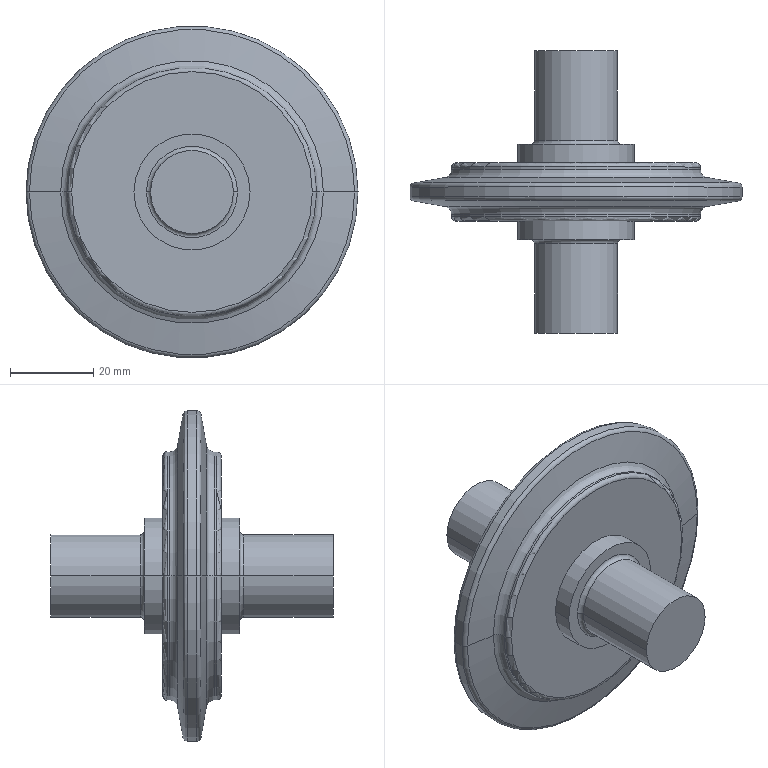Part | SolidWorks | features Revolution 1 | 1 solid | 40 faces | box 80 x 68 x 80 mm | volume 71844 mm3 | torus 16 | cylinder 14 | plane 6 | cone 4 | commonest cylinder face diameters 20 x4 28 x4 60 x4 80 x2
STEP:
#1=CARTESIAN_POINT('',(321.384,33.979,0.));
#2=VERTEX_POINT('',#1);
#3=CARTESIAN_POINT('',(258.079,33.979,0.));
#4=VERTEX_POINT('',#3);
#5=CARTESIAN_POINT('',(289.732,33.979,0.));
#6=DIRECTION('',(0.,-1.,0.));
#7=DIRECTION('',(1.,0.,0.));
#8=AXIS2_PLACEMENT_3D('',#5,#6,#7);
#9=CIRCLE('',#8,31.653);
#10=EDGE_CURVE('',#2,#4,#9,.T.);
#11=ORIENTED_EDGE('',*,*,#10,.T.);
#12=CARTESIAN_POINT('',(250.558,32.653,0.));
#13=VERTEX_POINT('',#12);
#14=CARTESIAN_POINT('',(258.079,33.979,0.));
#15=DIRECTION('',(-0.9848,-0.1736,0.));
#16=VECTOR('',#15,1000.);
#17=LINE('',#14,#16);
#18=EDGE_CURVE('',#4,#13,#17,.T.);
#19=ORIENTED_EDGE('',*,*,#18,.T.);
#20=CARTESIAN_POINT('',(328.905,32.653,0.));
#21=VERTEX_POINT('',#20);
#22=CARTESIAN_POINT('',(289.732,32.653,0.));
#23=DIRECTION('',(0.,-1.,0.));
#24=DIRECTION('',(1.,0.,0.));
#25=AXIS2_PLACEMENT_3D('',#22,#23,#24);
#26=CIRCLE('',#25,39.174);
#27=EDGE_CURVE('',#21,#13,#26,.T.);
#28=ORIENTED_EDGE('',*,*,#27,.F.);
#29=CARTESIAN_POINT('',(321.384,33.979,0.));
#30=DIRECTION('',(0.9848,-0.1736,0.));
#31=VECTOR('',#30,1000.);
#32=LINE('',#29,#31);
#33=EDGE_CURVE('',#2,#21,#32,.T.);
#34=ORIENTED_EDGE('',*,*,#33,.F.);
#35=EDGE_LOOP('',(#11,#19,#28,#34));
#36=FACE_OUTER_BOUND('',#35,.T.);
#37=CARTESIAN_POINT('',(289.732,33.979,0.));
#38=DIRECTION('',(0.,-1.,0.));
#39=DIRECTION('',(1.,0.,0.));
#40=AXIS2_PLACEMENT_3D('',#37,#38,#39);
#41=CONICAL_SURFACE('',#40,31.653,1.396);
#42=ADVANCED_FACE('',(#36),#41,.T.);
#43=CARTESIAN_POINT('',(289.732,33.979,0.));
#44=DIRECTION('',(0.,-1.,0.));
#45=DIRECTION('',(1.,0.,0.));
#46=AXIS2_PLACEMENT_3D('',#43,#44,#45);
#47=CIRCLE('',#46,31.653);
#48=EDGE_CURVE('',#4,#2,#47,.T.);
#49=ORIENTED_EDGE('',*,*,#48,.F.);
#50=CARTESIAN_POINT('',(259.732,35.948,0.));
#51=VERTEX_POINT('',#50);
#52=CARTESIAN_POINT('',(257.732,35.948,0.));
#53=DIRECTION('',(0.,0.,1.));
#54=DIRECTION('',(1.,0.,0.));
#55=AXIS2_PLACEMENT_3D('',#52,#53,#54);
#56=CIRCLE('',#55,2.);
#57=EDGE_CURVE('',#4,#51,#56,.T.);
#58=ORIENTED_EDGE('',*,*,#57,.T.);
#59=CARTESIAN_POINT('',(319.732,35.948,0.));
#60=VERTEX_POINT('',#59);
#61=CARTESIAN_POINT('',(289.732,35.948,0.));
#62=DIRECTION('',(0.,-1.,0.));
#63=DIRECTION('',(1.,0.,0.));
#64=AXIS2_PLACEMENT_3D('',#61,#62,#63);
#65=CIRCLE('',#64,30.);
#66=EDGE_CURVE('',#51,#60,#65,.T.);
#67=ORIENTED_EDGE('',*,*,#66,.T.);
#68=CARTESIAN_POINT('',(321.732,35.948,0.));
#69=DIRECTION('',(0.,0.,-1.));
#70=DIRECTION('',(-1.,0.,0.));
#71=AXIS2_PLACEMENT_3D('',#68,#69,#70);
#72=CIRCLE('',#71,2.);
#73=EDGE_CURVE('',#2,#60,#72,.T.);
#74=ORIENTED_EDGE('',*,*,#73,.F.);
#75=EDGE_LOOP('',(#49,#58,#67,#74));
#76=FACE_OUTER_BOUND('',#75,.T.);
#77=CARTESIAN_POINT('',(289.732,35.948,0.));
#78=DIRECTION('',(0.,-1.,0.));
#79=DIRECTION('',(1.,0.,0.));
#80=AXIS2_PLACEMENT_3D('',#77,#78,#79);
#81=TOROIDAL_SURFACE('',#80,32.,2.);
#82=ADVANCED_FACE('',(#76),#81,.F.);
#83=CARTESIAN_POINT('',(319.732,36.507,0.));
#84=VERTEX_POINT('',#83);
#85=CARTESIAN_POINT('',(259.732,36.507,0.));
#86=VERTEX_POINT('',#85);
#87=CARTESIAN_POINT('',(289.732,36.507,0.));
#88=DIRECTION('',(0.,-1.,0.));
#89=DIRECTION('',(1.,0.,0.));
#90=AXIS2_PLACEMENT_3D('',#87,#88,#89);
#91=CIRCLE('',#90,30.);
#92=EDGE_CURVE('',#84,#86,#91,.T.);
#93=ORIENTED_EDGE('',*,*,#92,.T.);
#94=CARTESIAN_POINT('',(259.732,-3.493,0.));
#95=DIRECTION('',(0.,-1.,0.));
#96=VECTOR('',#95,1000.);
#97=LINE('',#94,#96);
#98=EDGE_CURVE('',#86,#51,#97,.T.);
#99=ORIENTED_EDGE('',*,*,#98,.T.);
#100=CARTESIAN_POINT('',(289.732,35.948,0.));
#101=DIRECTION('',(0.,-1.,0.));
#102=DIRECTION('',(1.,0.,0.));
#103=AXIS2_PLACEMENT_3D('',#100,#101,#102);
#104=CIRCLE('',#103,30.);
#105=EDGE_CURVE('',#60,#51,#104,.T.);
#106=ORIENTED_EDGE('',*,*,#105,.F.);
#107=CARTESIAN_POINT('',(319.732,-3.493,0.));
#108=DIRECTION('',(0.,-1.,0.));
#109=VECTOR('',#108,1000.);
#110=LINE('',#107,#109);
#111=EDGE_CURVE('',#84,#60,#110,.T.);
#112=ORIENTED_EDGE('',*,*,#111,.F.);
#113=EDGE_LOOP('',(#93,#99,#106,#112));
#114=FACE_OUTER_BOUND('',#113,.T.);
#115=CARTESIAN_POINT('',(289.732,-3.493,0.));
#116=DIRECTION('',(0.,-1.,0.));
#117=DIRECTION('',(1.,0.,0.));
#118=AXIS2_PLACEMENT_3D('',#115,#116,#117);
#119=CYLINDRICAL_SURFACE('',#118,30.);
#120=ADVANCED_FACE('',(#114),#119,.T.);
#121=CARTESIAN_POINT('',(318.732,37.507,0.));
#122=VERTEX_POINT('',#121);
#123=CARTESIAN_POINT('',(260.732,37.507,0.));
#124=VERTEX_POINT('',#123);
#125=CARTESIAN_POINT('',(289.732,37.507,0.));
#126=DIRECTION('',(0.,-1.,0.));
#127=DIRECTION('',(1.,0.,0.));
#128=AXIS2_PLACEMENT_3D('',#125,#126,#127);
#129=CIRCLE('',#128,29.);
#130=EDGE_CURVE('',#122,#124,#129,.T.);
#131=ORIENTED_EDGE('',*,*,#130,.T.);
#132=CARTESIAN_POINT('',(260.732,36.507,0.));
#133=DIRECTION('',(0.,0.,1.));
#134=DIRECTION('',(1.,0.,0.));
#135=AXIS2_PLACEMENT_3D('',#132,#133,#134);
#136=CIRCLE('',#135,1.);
#137=EDGE_CURVE('',#124,#86,#136,.T.);
#138=ORIENTED_EDGE('',*,*,#137,.T.);
#139=ORIENTED_EDGE('',*,*,#92,.F.);
#140=CARTESIAN_POINT('',(318.732,36.507,0.));
#141=DIRECTION('',(0.,0.,-1.));
#142=DIRECTION('',(-1.,0.,0.));
#143=AXIS2_PLACEMENT_3D('',#140,#141,#142);
#144=CIRCLE('',#143,1.);
#145=EDGE_CURVE('',#122,#84,#144,.T.);
#146=ORIENTED_EDGE('',*,*,#145,.F.);
#147=EDGE_LOOP('',(#131,#138,#139,#146));
#148=FACE_OUTER_BOUND('',#147,.T.);
#149=CARTESIAN_POINT('',(289.732,36.507,0.));
#150=DIRECTION('',(0.,-1.,0.));
#151=DIRECTION('',(1.,0.,0.));
#152=AXIS2_PLACEMENT_3D('',#149,#150,#151);
#153=TOROIDAL_SURFACE('',#152,29.,1.);
#154=ADVANCED_FACE('',(#148),#153,.T.);
#155=CARTESIAN_POINT('',(303.732,42.007,0.));
#156=VERTEX_POINT('',#155);
#157=CARTESIAN_POINT('',(275.732,42.007,0.));
#158=VERTEX_POINT('',#157);
#159=CARTESIAN_POINT('',(289.732,42.007,0.));
#160=DIRECTION('',(0.,-1.,0.));
#161=DIRECTION('',(1.,0.,0.));
#162=AXIS2_PLACEMENT_3D('',#159,#160,#161);
#163=CIRCLE('',#162,14.);
#164=EDGE_CURVE('',#156,#158,#163,.T.);
#165=ORIENTED_EDGE('',*,*,#164,.T.);
#166=CARTESIAN_POINT('',(275.732,37.507,0.));
#167=VERTEX_POINT('',#166);
#168=CARTESIAN_POINT('',(275.732,-3.493,0.));
#169=DIRECTION('',(0.,-1.,0.));
#170=VECTOR('',#169,1000.);
#171=LINE('',#168,#170);
#172=EDGE_CURVE('',#158,#167,#171,.T.);
#173=ORIENTED_EDGE('',*,*,#172,.T.);
#174=CARTESIAN_POINT('',(303.732,37.507,0.));
#175=VERTEX_POINT('',#174);
#176=CARTESIAN_POINT('',(289.732,37.507,0.));
#177=DIRECTION('',(0.,-1.,0.));
#178=DIRECTION('',(1.,0.,0.));
#179=AXIS2_PLACEMENT_3D('',#176,#177,#178);
#180=CIRCLE('',#179,14.);
#181=EDGE_CURVE('',#175,#167,#180,.T.);
#182=ORIENTED_EDGE('',*,*,#181,.F.);
#183=CARTESIAN_POINT('',(303.732,-3.493,0.));
#184=DIRECTION('',(0.,-1.,0.));
#185=VECTOR('',#184,1000.);
#186=LINE('',#183,#185);
#187=EDGE_CURVE('',#156,#175,#186,.T.);
#188=ORIENTED_EDGE('',*,*,#187,.F.);
#189=EDGE_LOOP('',(#165,#173,#182,#188));
#190=FACE_OUTER_BOUND('',#189,.T.);
#191=CARTESIAN_POINT('',(289.732,-3.493,0.));
#192=DIRECTION('',(0.,-1.,0.));
#193=DIRECTION('',(1.,0.,0.));
#194=AXIS2_PLACEMENT_3D('',#191,#192,#193);
#195=CYLINDRICAL_SURFACE('',#194,14.);
#196=ADVANCED_FACE('',(#190),#195,.T.);
#197=CARTESIAN_POINT('',(278.732,42.007,0.));
#198=VERTEX_POINT('',#197);
#199=CARTESIAN_POINT('',(300.732,42.007,0.));
#200=VERTEX_POINT('',#199);
#201=CARTESIAN_POINT('',(289.732,42.007,0.));
#202=DIRECTION('',(0.,-1.,0.));
#203=DIRECTION('',(1.,0.,0.));
#204=AXIS2_PLACEMENT_3D('',#201,#202,#203);
#205=CIRCLE('',#204,11.);
#206=EDGE_CURVE('',#198,#200,#205,.T.);
#207=ORIENTED_EDGE('',*,*,#206,.F.);
#208=CARTESIAN_POINT('',(279.732,43.007,0.));
#209=VERTEX_POINT('',#208);
#210=CARTESIAN_POINT('',(278.732,43.007,0.));
#211=DIRECTION('',(0.,0.,1.));
#212=DIRECTION('',(1.,0.,0.));
#213=AXIS2_PLACEMENT_3D('',#210,#211,#212);
#214=CIRCLE('',#213,1.);
#215=EDGE_CURVE('',#198,#209,#214,.T.);
#216=ORIENTED_EDGE('',*,*,#215,.T.);
#217=CARTESIAN_POINT('',(299.732,43.007,0.));
#218=VERTEX_POINT('',#217);
#219=CARTESIAN_POINT('',(289.732,43.007,0.));
#220=DIRECTION('',(0.,-1.,0.));
#221=DIRECTION('',(1.,0.,0.));
#222=AXIS2_PLACEMENT_3D('',#219,#220,#221);
#223=CIRCLE('',#222,10.);
#224=EDGE_CURVE('',#209,#218,#223,.T.);
#225=ORIENTED_EDGE('',*,*,#224,.T.);
#226=CARTESIAN_POINT('',(300.732,43.007,0.));
#227=DIRECTION('',(0.,0.,-1.));
#228=DIRECTION('',(-1.,0.,0.));
#229=AXIS2_PLACEMENT_3D('',#226,#227,#228);
#230=CIRCLE('',#229,1.);
#231=EDGE_CURVE('',#200,#218,#230,.T.);
#232=ORIENTED_EDGE('',*,*,#231,.F.);
#233=EDGE_LOOP('',(#207,#216,#225,#232));
#234=FACE_OUTER_BOUND('',#233,.T.);
#235=CARTESIAN_POINT('',(289.732,43.007,0.));
#236=DIRECTION('',(0.,-1.,0.));
#237=DIRECTION('',(1.,0.,0.));
#238=AXIS2_PLACEMENT_3D('',#235,#236,#237);
#239=TOROIDAL_SURFACE('',#238,11.,1.);
#240=ADVANCED_FACE('',(#234),#239,.F.);
#241=CARTESIAN_POINT('',(299.732,64.507,0.));
#242=VERTEX_POINT('',#241);
#243=CARTESIAN_POINT('',(279.732,64.507,0.));
#244=VERTEX_POINT('',#243);
#245=CARTESIAN_POINT('',(289.732,64.507,0.));
#246=DIRECTION('',(0.,-1.,0.));
#247=DIRECTION('',(1.,0.,0.));
#248=AXIS2_PLACEMENT_3D('',#245,#246,#247);
#249=CIRCLE('',#248,10.);
#250=EDGE_CURVE('',#242,#244,#249,.T.);
#251=ORIENTED_EDGE('',*,*,#250,.T.);
#252=CARTESIAN_POINT('',(279.732,-3.493,0.));
#253=DIRECTION('',(0.,-1.,0.));
#254=VECTOR('',#253,1000.);
#255=LINE('',#252,#254);
#256=EDGE_CURVE('',#244,#209,#255,.T.);
#257=ORIENTED_EDGE('',*,*,#256,.T.);
#258=CARTESIAN_POINT('',(289.732,43.007,0.));
#259=DIRECTION('',(0.,-1.,0.));
#260=DIRECTION('',(1.,0.,0.));
#261=AXIS2_PLACEMENT_3D('',#258,#259,#260);
#262=CIRCLE('',#261,10.);
#263=EDGE_CURVE('',#218,#209,#262,.T.);
#264=ORIENTED_EDGE('',*,*,#263,.F.);
#265=CARTESIAN_POINT('',(299.732,-3.493,0.));
#266=DIRECTION('',(0.,-1.,0.));
#267=VECTOR('',#266,1000.);
#268=LINE('',#265,#267);
#269=EDGE_CURVE('',#242,#218,#268,.T.);
#270=ORIENTED_EDGE('',*,*,#269,.F.);
#271=EDGE_LOOP('',(#251,#257,#264,#270));
#272=FACE_OUTER_BOUND('',#271,.T.);
#273=CARTESIAN_POINT('',(289.732,-3.493,0.));
#274=DIRECTION('',(0.,-1.,0.));
#275=DIRECTION('',(1.,0.,0.));
#276=AXIS2_PLACEMENT_3D('',#273,#274,#275);
#277=CYLINDRICAL_SURFACE('',#276,10.);
#278=ADVANCED_FACE('',(#272),#277,.T.);
#279=CARTESIAN_POINT('',(299.732,18.007,0.));
#280=VERTEX_POINT('',#279);
#281=CARTESIAN_POINT('',(279.732,18.007,0.));
#282=VERTEX_POINT('',#281);
#283=CARTESIAN_POINT('',(289.732,18.007,0.));
#284=DIRECTION('',(0.,-1.,0.));
#285=DIRECTION('',(1.,0.,0.));
#286=AXIS2_PLACEMENT_3D('',#283,#284,#285);
#287=CIRCLE('',#286,10.);
#288=EDGE_CURVE('',#280,#282,#287,.T.);
#289=ORIENTED_EDGE('',*,*,#288,.T.);
#290=CARTESIAN_POINT('',(279.732,-3.493,0.));
#291=VERTEX_POINT('',#290);
#292=CARTESIAN_POINT('',(279.732,-3.493,0.));
#293=DIRECTION('',(0.,-1.,0.));
#294=VECTOR('',#293,1000.);
#295=LINE('',#292,#294);
#296=EDGE_CURVE('',#282,#291,#295,.T.);
#297=ORIENTED_EDGE('',*,*,#296,.T.);
#298=CARTESIAN_POINT('',(299.732,-3.493,0.));
#299=VERTEX_POINT('',#298);
#300=CARTESIAN_POINT('',(289.732,-3.493,0.));
#301=DIRECTION('',(0.,-1.,0.));
#302=DIRECTION('',(1.,0.,0.));
#303=AXIS2_PLACEMENT_3D('',#300,#301,#302);
#304=CIRCLE('',#303,10.);
#305=EDGE_CURVE('',#299,#291,#304,.T.);
#306=ORIENTED_EDGE('',*,*,#305,.F.);
#307=CARTESIAN_POINT('',(299.732,-3.493,0.));
#308=DIRECTION('',(0.,-1.,0.));
#309=VECTOR('',#308,1000.);
#310=LINE('',#307,#309);
#311=EDGE_CURVE('',#280,#299,#310,.T.);
#312=ORIENTED_EDGE('',*,*,#311,.F.);
#313=EDGE_LOOP('',(#289,#297,#306,#312));
#314=FACE_OUTER_BOUND('',#313,.T.);
#315=CARTESIAN_POINT('',(289.732,-3.493,0.));
#316=DIRECTION('',(0.,-1.,0.));
#317=DIRECTION('',(1.,0.,0.));
#318=AXIS2_PLACEMENT_3D('',#315,#316,#317);
#319=CYLINDRICAL_SURFACE('',#318,10.);
#320=ADVANCED_FACE('',(#314),#319,.T.);
#321=CARTESIAN_POINT('',(289.732,18.007,0.));
#322=DIRECTION('',(0.,-1.,0.));
#323=DIRECTION('',(1.,0.,0.));
#324=AXIS2_PLACEMENT_3D('',#321,#322,#323);
#325=CIRCLE('',#324,10.);
#326=EDGE_CURVE('',#282,#280,#325,.T.);
#327=ORIENTED_EDGE('',*,*,#326,.F.);
#328=CARTESIAN_POINT('',(278.732,19.007,0.));
#329=VERTEX_POINT('',#328);
#330=CARTESIAN_POINT('',(278.732,18.007,0.));
#331=DIRECTION('',(0.,0.,1.));
#332=DIRECTION('',(1.,0.,0.));
#333=AXIS2_PLACEMENT_3D('',#330,#331,#332);
#334=CIRCLE('',#333,1.);
#335=EDGE_CURVE('',#282,#329,#334,.T.);
#336=ORIENTED_EDGE('',*,*,#335,.T.);
#337=CARTESIAN_POINT('',(300.732,19.007,0.));
#338=VERTEX_POINT('',#337);
#339=CARTESIAN_POINT('',(289.732,19.007,0.));
#340=DIRECTION('',(0.,-1.,0.));
#341=DIRECTION('',(1.,0.,0.));
#342=AXIS2_PLACEMENT_3D('',#339,#340,#341);
#343=CIRCLE('',#342,11.);
#344=EDGE_CURVE('',#329,#338,#343,.T.);
#345=ORIENTED_EDGE('',*,*,#344,.T.);
#346=CARTESIAN_POINT('',(300.732,18.007,0.));
#347=DIRECTION('',(0.,0.,-1.));
#348=DIRECTION('',(-1.,0.,0.));
#349=AXIS2_PLACEMENT_3D('',#346,#347,#348);
#350=CIRCLE('',#349,1.);
#351=EDGE_CURVE('',#280,#338,#350,.T.);
#352=ORIENTED_EDGE('',*,*,#351,.F.);
#353=EDGE_LOOP('',(#327,#336,#345,#352));
#354=FACE_OUTER_BOUND('',#353,.T.);
#355=CARTESIAN_POINT('',(289.732,18.007,0.));
#356=DIRECTION('',(0.,-1.,0.));
#357=DIRECTION('',(1.,0.,0.));
#358=AXIS2_PLACEMENT_3D('',#355,#356,#357);
#359=TOROIDAL_SURFACE('',#358,11.,1.);
#360=ADVANCED_FACE('',(#354),#359,.F.);
#361=CARTESIAN_POINT('',(303.732,23.507,0.));
#362=VERTEX_POINT('',#361);
#363=CARTESIAN_POINT('',(275.732,23.507,0.));
#364=VERTEX_POINT('',#363);
#365=CARTESIAN_POINT('',(289.732,23.507,0.));
#366=DIRECTION('',(0.,-1.,0.));
#367=DIRECTION('',(1.,0.,0.));
#368=AXIS2_PLACEMENT_3D('',#365,#366,#367);
#369=CIRCLE('',#368,14.);
#370=EDGE_CURVE('',#362,#364,#369,.T.);
#371=ORIENTED_EDGE('',*,*,#370,.T.);
#372=CARTESIAN_POINT('',(275.732,19.007,0.));
#373=VERTEX_POINT('',#372);
#374=CARTESIAN_POINT('',(275.732,-3.493,0.));
#375=DIRECTION('',(0.,-1.,0.));
#376=VECTOR('',#375,1000.);
#377=LINE('',#374,#376);
#378=EDGE_CURVE('',#364,#373,#377,.T.);
#379=ORIENTED_EDGE('',*,*,#378,.T.);
#380=CARTESIAN_POINT('',(303.732,19.007,0.));
#381=VERTEX_POINT('',#380);
#382=CARTESIAN_POINT('',(289.732,19.007,0.));
#383=DIRECTION('',(0.,-1.,0.));
#384=DIRECTION('',(1.,0.,0.));
#385=AXIS2_PLACEMENT_3D('',#382,#383,#384);
#386=CIRCLE('',#385,14.);
#387=EDGE_CURVE('',#381,#373,#386,.T.);
#388=ORIENTED_EDGE('',*,*,#387,.F.);
#389=CARTESIAN_POINT('',(303.732,-3.493,0.));
#390=DIRECTION('',(0.,-1.,0.));
#391=VECTOR('',#390,1000.);
#392=LINE('',#389,#391);
#393=EDGE_CURVE('',#362,#381,#392,.T.);
#394=ORIENTED_EDGE('',*,*,#393,.F.);
#395=EDGE_LOOP('',(#371,#379,#388,#394));
#396=FACE_OUTER_BOUND('',#395,.T.);
#397=CARTESIAN_POINT('',(289.732,-3.493,0.));
#398=DIRECTION('',(0.,-1.,0.));
#399=DIRECTION('',(1.,0.,0.));
#400=AXIS2_PLACEMENT_3D('',#397,#398,#399);
#401=CYLINDRICAL_SURFACE('',#400,14.);
#402=ADVANCED_FACE('',(#396),#401,.T.);
#403=CARTESIAN_POINT('',(319.732,24.507,0.));
#404=VERTEX_POINT('',#403);
#405=CARTESIAN_POINT('',(259.732,24.507,0.));
#406=VERTEX_POINT('',#405);
#407=CARTESIAN_POINT('',(289.732,24.507,0.));
#408=DIRECTION('',(0.,-1.,0.));
#409=DIRECTION('',(1.,0.,0.));
#410=AXIS2_PLACEMENT_3D('',#407,#408,#409);
#411=CIRCLE('',#410,30.);
#412=EDGE_CURVE('',#404,#406,#411,.T.);
#413=ORIENTED_EDGE('',*,*,#412,.T.);
#414=CARTESIAN_POINT('',(260.732,23.507,0.));
#415=VERTEX_POINT('',#414);
#416=CARTESIAN_POINT('',(260.732,24.507,0.));
#417=DIRECTION('',(0.,0.,1.));
#418=DIRECTION('',(1.,0.,0.));
#419=AXIS2_PLACEMENT_3D('',#416,#417,#418);
#420=CIRCLE('',#419,1.);
#421=EDGE_CURVE('',#406,#415,#420,.T.);
#422=ORIENTED_EDGE('',*,*,#421,.T.);
#423=CARTESIAN_POINT('',(318.732,23.507,0.));
#424=VERTEX_POINT('',#423);
#425=CARTESIAN_POINT('',(289.732,23.507,0.));
#426=DIRECTION('',(0.,-1.,0.));
#427=DIRECTION('',(1.,0.,0.));
#428=AXIS2_PLACEMENT_3D('',#425,#426,#427);
#429=CIRCLE('',#428,29.);
#430=EDGE_CURVE('',#424,#415,#429,.T.);
#431=ORIENTED_EDGE('',*,*,#430,.F.);
#432=CARTESIAN_POINT('',(318.732,24.507,0.));
#433=DIRECTION('',(0.,0.,-1.));
#434=DIRECTION('',(-1.,0.,0.));
#435=AXIS2_PLACEMENT_3D('',#432,#433,#434);
#436=CIRCLE('',#435,1.);
#437=EDGE_CURVE('',#404,#424,#436,.T.);
#438=ORIENTED_EDGE('',*,*,#437,.F.);
#439=EDGE_LOOP('',(#413,#422,#431,#438));
#440=FACE_OUTER_BOUND('',#439,.T.);
#441=CARTESIAN_POINT('',(289.732,24.507,0.));
#442=DIRECTION('',(0.,-1.,0.));
#443=DIRECTION('',(1.,0.,0.));
#444=AXIS2_PLACEMENT_3D('',#441,#442,#443);
#445=TOROIDAL_SURFACE('',#444,29.,1.);
#446=ADVANCED_FACE('',(#440),#445,.T.);
#447=CARTESIAN_POINT('',(319.732,25.065,0.));
#448=VERTEX_POINT('',#447);
#449=CARTESIAN_POINT('',(259.732,25.065,0.));
#450=VERTEX_POINT('',#449);
#451=CARTESIAN_POINT('',(289.732,25.065,0.));
#452=DIRECTION('',(0.,-1.,0.));
#453=DIRECTION('',(1.,0.,0.));
#454=AXIS2_PLACEMENT_3D('',#451,#452,#453);
#455=CIRCLE('',#454,30.);
#456=EDGE_CURVE('',#448,#450,#455,.T.);
#457=ORIENTED_EDGE('',*,*,#456,.T.);
#458=CARTESIAN_POINT('',(259.732,-3.493,0.));
#459=DIRECTION('',(0.,-1.,0.));
#460=VECTOR('',#459,1000.);
#461=LINE('',#458,#460);
#462=EDGE_CURVE('',#450,#406,#461,.T.);
#463=ORIENTED_EDGE('',*,*,#462,.T.);
#464=ORIENTED_EDGE('',*,*,#412,.F.);
#465=CARTESIAN_POINT('',(319.732,-3.493,0.));
#466=DIRECTION('',(0.,-1.,0.));
#467=VECTOR('',#466,1000.);
#468=LINE('',#465,#467);
#469=EDGE_CURVE('',#448,#404,#468,.T.);
#470=ORIENTED_EDGE('',*,*,#469,.F.);
#471=EDGE_LOOP('',(#457,#463,#464,#470));
#472=FACE_OUTER_BOUND('',#471,.T.);
#473=CARTESIAN_POINT('',(289.732,-3.493,0.));
#474=DIRECTION('',(0.,-1.,0.));
#475=DIRECTION('',(1.,0.,0.));
#476=AXIS2_PLACEMENT_3D('',#473,#474,#475);
#477=CYLINDRICAL_SURFACE('',#476,30.);
#478=ADVANCED_FACE('',(#472),#477,.T.);
#479=CARTESIAN_POINT('',(289.732,25.065,0.));
#480=DIRECTION('',(0.,-1.,0.));
#481=DIRECTION('',(1.,0.,0.));
#482=AXIS2_PLACEMENT_3D('',#479,#480,#481);
#483=CIRCLE('',#482,30.);
#484=EDGE_CURVE('',#450,#448,#483,.T.);
#485=ORIENTED_EDGE('',*,*,#484,.F.);
#486=CARTESIAN_POINT('',(258.079,27.035,0.));
#487=VERTEX_POINT('',#486);
#488=CARTESIAN_POINT('',(257.732,25.065,0.));
#489=DIRECTION('',(0.,0.,1.));
#490=DIRECTION('',(1.,0.,0.));
#491=AXIS2_PLACEMENT_3D('',#488,#489,#490);
#492=CIRCLE('',#491,2.);
#493=EDGE_CURVE('',#450,#487,#492,.T.);
#494=ORIENTED_EDGE('',*,*,#493,.T.);
#495=CARTESIAN_POINT('',(321.384,27.035,0.));
#496=VERTEX_POINT('',#495);
#497=CARTESIAN_POINT('',(289.732,27.035,0.));
#498=DIRECTION('',(0.,-1.,0.));
#499=DIRECTION('',(1.,0.,0.));
#500=AXIS2_PLACEMENT_3D('',#497,#498,#499);
#501=CIRCLE('',#500,31.653);
#502=EDGE_CURVE('',#487,#496,#501,.T.);
#503=ORIENTED_EDGE('',*,*,#502,.T.);
#504=CARTESIAN_POINT('',(321.732,25.065,0.));
#505=DIRECTION('',(0.,0.,-1.));
#506=DIRECTION('',(-1.,0.,0.));
#507=AXIS2_PLACEMENT_3D('',#504,#505,#506);
#508=CIRCLE('',#507,2.);
#509=EDGE_CURVE('',#448,#496,#508,.T.);
#510=ORIENTED_EDGE('',*,*,#509,.F.);
#511=EDGE_LOOP('',(#485,#494,#503,#510));
#512=FACE_OUTER_BOUND('',#511,.T.);
#513=CARTESIAN_POINT('',(289.732,25.065,0.));
#514=DIRECTION('',(0.,-1.,0.));
#515=DIRECTION('',(1.,0.,0.));
#516=AXIS2_PLACEMENT_3D('',#513,#514,#515);
#517=TOROIDAL_SURFACE('',#516,32.,2.);
#518=ADVANCED_FACE('',(#512),#517,.F.);
#519=CARTESIAN_POINT('',(289.732,27.035,0.));
#520=DIRECTION('',(0.,-1.,0.));
#521=DIRECTION('',(1.,0.,0.));
#522=AXIS2_PLACEMENT_3D('',#519,#520,#521);
#523=CIRCLE('',#522,31.653);
#524=EDGE_CURVE('',#496,#487,#523,.T.);
#525=ORIENTED_EDGE('',*,*,#524,.F.);
#526=CARTESIAN_POINT('',(328.905,28.361,0.));
#527=VERTEX_POINT('',#526);
#528=CARTESIAN_POINT('',(328.905,28.361,0.));
#529=DIRECTION('',(0.9848,0.1736,0.));
#530=VECTOR('',#529,1000.);
#531=LINE('',#528,#530);
#532=EDGE_CURVE('',#496,#527,#531,.T.);
#533=ORIENTED_EDGE('',*,*,#532,.T.);
#534=CARTESIAN_POINT('',(250.558,28.361,0.));
#535=VERTEX_POINT('',#534);
#536=CARTESIAN_POINT('',(289.732,28.361,0.));
#537=DIRECTION('',(0.,-1.,0.));
#538=DIRECTION('',(1.,0.,0.));
#539=AXIS2_PLACEMENT_3D('',#536,#537,#538);
#540=CIRCLE('',#539,39.174);
#541=EDGE_CURVE('',#527,#535,#540,.T.);
#542=ORIENTED_EDGE('',*,*,#541,.T.);
#543=CARTESIAN_POINT('',(250.558,28.361,0.));
#544=DIRECTION('',(-0.9848,0.1736,0.));
#545=VECTOR('',#544,1000.);
#546=LINE('',#543,#545);
#547=EDGE_CURVE('',#487,#535,#546,.T.);
#548=ORIENTED_EDGE('',*,*,#547,.F.);
#549=EDGE_LOOP('',(#525,#533,#542,#548));
#550=FACE_OUTER_BOUND('',#549,.T.);
#551=CARTESIAN_POINT('',(289.732,28.361,0.));
#552=DIRECTION('',(0.,1.,0.));
#553=DIRECTION('',(-1.,0.,0.));
#554=AXIS2_PLACEMENT_3D('',#551,#552,#553);
#555=CONICAL_SURFACE('',#554,39.174,1.396);
#556=ADVANCED_FACE('',(#550),#555,.T.);
#557=CARTESIAN_POINT('',(329.732,29.346,0.));
#558=VERTEX_POINT('',#557);
#559=CARTESIAN_POINT('',(249.732,29.346,0.));
#560=VERTEX_POINT('',#559);
#561=CARTESIAN_POINT('',(289.732,29.346,0.));
#562=DIRECTION('',(0.,-1.,0.));
#563=DIRECTION('',(1.,0.,0.));
#564=AXIS2_PLACEMENT_3D('',#561,#562,#563);
#565=CIRCLE('',#564,40.);
#566=EDGE_CURVE('',#558,#560,#565,.T.);
#567=ORIENTED_EDGE('',*,*,#566,.T.);
#568=CARTESIAN_POINT('',(250.732,29.346,0.));
#569=DIRECTION('',(0.,0.,1.));
#570=DIRECTION('',(1.,0.,0.));
#571=AXIS2_PLACEMENT_3D('',#568,#569,#570);
#572=CIRCLE('',#571,1.);
#573=EDGE_CURVE('',#560,#535,#572,.T.);
#574=ORIENTED_EDGE('',*,*,#573,.T.);
#575=ORIENTED_EDGE('',*,*,#541,.F.);
#576=CARTESIAN_POINT('',(328.732,29.346,0.));
#577=DIRECTION('',(0.,0.,-1.));
#578=DIRECTION('',(-1.,0.,0.));
#579=AXIS2_PLACEMENT_3D('',#576,#577,#578);
#580=CIRCLE('',#579,1.);
#581=EDGE_CURVE('',#558,#527,#580,.T.);
#582=ORIENTED_EDGE('',*,*,#581,.F.);
#583=EDGE_LOOP('',(#567,#574,#575,#582));
#584=FACE_OUTER_BOUND('',#583,.T.);
#585=CARTESIAN_POINT('',(289.732,29.346,0.));
#586=DIRECTION('',(0.,-1.,0.));
#587=DIRECTION('',(1.,0.,0.));
#588=AXIS2_PLACEMENT_3D('',#585,#586,#587);
#589=TOROIDAL_SURFACE('',#588,39.,1.);
#590=ADVANCED_FACE('',(#584),#589,.T.);
#591=CARTESIAN_POINT('',(329.732,31.668,0.));
#592=VERTEX_POINT('',#591);
#593=CARTESIAN_POINT('',(249.732,31.668,0.));
#594=VERTEX_POINT('',#593);
#595=CARTESIAN_POINT('',(289.732,31.668,0.));
#596=DIRECTION('',(0.,-1.,0.));
#597=DIRECTION('',(1.,0.,0.));
#598=AXIS2_PLACEMENT_3D('',#595,#596,#597);
#599=CIRCLE('',#598,40.);
#600=EDGE_CURVE('',#592,#594,#599,.T.);
#601=ORIENTED_EDGE('',*,*,#600,.T.);
#602=CARTESIAN_POINT('',(249.732,-3.493,0.));
#603=DIRECTION('',(0.,-1.,0.));
#604=VECTOR('',#603,1000.);
#605=LINE('',#602,#604);
#606=EDGE_CURVE('',#594,#560,#605,.T.);
#607=ORIENTED_EDGE('',*,*,#606,.T.);
#608=ORIENTED_EDGE('',*,*,#566,.F.);
#609=CARTESIAN_POINT('',(329.732,-3.493,0.));
#610=DIRECTION('',(0.,-1.,0.));
#611=VECTOR('',#610,1000.);
#612=LINE('',#609,#611);
#613=EDGE_CURVE('',#592,#558,#612,.T.);
#614=ORIENTED_EDGE('',*,*,#613,.F.);
#615=EDGE_LOOP('',(#601,#607,#608,#614));
#616=FACE_OUTER_BOUND('',#615,.T.);
#617=CARTESIAN_POINT('',(289.732,-3.493,0.));
#618=DIRECTION('',(0.,-1.,0.));
#619=DIRECTION('',(1.,0.,0.));
#620=AXIS2_PLACEMENT_3D('',#617,#618,#619);
#621=CYLINDRICAL_SURFACE('',#620,40.);
#622=ADVANCED_FACE('',(#616),#621,.T.);
#623=ORIENTED_EDGE('',*,*,#27,.T.);
#624=CARTESIAN_POINT('',(250.732,31.668,0.));
#625=DIRECTION('',(0.,0.,1.));
#626=DIRECTION('',(1.,0.,0.));
#627=AXIS2_PLACEMENT_3D('',#624,#625,#626);
#628=CIRCLE('',#627,1.);
#629=EDGE_CURVE('',#13,#594,#628,.T.);
#630=ORIENTED_EDGE('',*,*,#629,.T.);
#631=ORIENTED_EDGE('',*,*,#600,.F.);
#632=CARTESIAN_POINT('',(328.732,31.668,0.));
#633=DIRECTION('',(0.,0.,-1.));
#634=DIRECTION('',(-1.,0.,0.));
#635=AXIS2_PLACEMENT_3D('',#632,#633,#634);
#636=CIRCLE('',#635,1.);
#637=EDGE_CURVE('',#21,#592,#636,.T.);
#638=ORIENTED_EDGE('',*,*,#637,.F.);
#639=EDGE_LOOP('',(#623,#630,#631,#638));
#640=FACE_OUTER_BOUND('',#639,.T.);
#641=CARTESIAN_POINT('',(289.732,31.668,0.));
#642=DIRECTION('',(0.,-1.,0.));
#643=DIRECTION('',(1.,0.,0.));
#644=AXIS2_PLACEMENT_3D('',#641,#642,#643);
#645=TOROIDAL_SURFACE('',#644,39.,1.);
#646=ADVANCED_FACE('',(#640),#645,.T.);
#647=ORIENTED_EDGE('',*,*,#629,.F.);
#648=CARTESIAN_POINT('',(289.732,32.653,0.));
#649=DIRECTION('',(0.,-1.,0.));
#650=DIRECTION('',(1.,0.,0.));
#651=AXIS2_PLACEMENT_3D('',#648,#649,#650);
#652=CIRCLE('',#651,39.174);
#653=EDGE_CURVE('',#13,#21,#652,.T.);
#654=ORIENTED_EDGE('',*,*,#653,.T.);
#655=ORIENTED_EDGE('',*,*,#637,.T.);
#656=CARTESIAN_POINT('',(289.732,31.668,0.));
#657=DIRECTION('',(0.,-1.,0.));
#658=DIRECTION('',(1.,0.,0.));
#659=AXIS2_PLACEMENT_3D('',#656,#657,#658);
#660=CIRCLE('',#659,40.);
#661=EDGE_CURVE('',#594,#592,#660,.T.);
#662=ORIENTED_EDGE('',*,*,#661,.F.);
#663=EDGE_LOOP('',(#647,#654,#655,#662));
#664=FACE_OUTER_BOUND('',#663,.T.);
#665=CARTESIAN_POINT('',(289.732,31.668,0.));
#666=DIRECTION('',(0.,-1.,0.));
#667=DIRECTION('',(1.,0.,0.));
#668=AXIS2_PLACEMENT_3D('',#665,#666,#667);
#669=TOROIDAL_SURFACE('',#668,39.,1.);
#670=ADVANCED_FACE('',(#664),#669,.T.);
#671=ORIENTED_EDGE('',*,*,#606,.F.);
#672=ORIENTED_EDGE('',*,*,#661,.T.);
#673=ORIENTED_EDGE('',*,*,#613,.T.);
#674=CARTESIAN_POINT('',(289.732,29.346,0.));
#675=DIRECTION('',(0.,-1.,0.));
#676=DIRECTION('',(1.,0.,0.));
#677=AXIS2_PLACEMENT_3D('',#674,#675,#676);
#678=CIRCLE('',#677,40.);
#679=EDGE_CURVE('',#560,#558,#678,.T.);
#680=ORIENTED_EDGE('',*,*,#679,.F.);
#681=EDGE_LOOP('',(#671,#672,#673,#680));
#682=FACE_OUTER_BOUND('',#681,.T.);
#683=CARTESIAN_POINT('',(289.732,-3.493,0.));
#684=DIRECTION('',(0.,-1.,0.));
#685=DIRECTION('',(1.,0.,0.));
#686=AXIS2_PLACEMENT_3D('',#683,#684,#685);
#687=CYLINDRICAL_SURFACE('',#686,40.);
#688=ADVANCED_FACE('',(#682),#687,.T.);
#689=ORIENTED_EDGE('',*,*,#573,.F.);
#690=ORIENTED_EDGE('',*,*,#679,.T.);
#691=ORIENTED_EDGE('',*,*,#581,.T.);
#692=CARTESIAN_POINT('',(289.732,28.361,0.));
#693=DIRECTION('',(0.,-1.,0.));
#694=DIRECTION('',(1.,0.,0.));
#695=AXIS2_PLACEMENT_3D('',#692,#693,#694);
#696=CIRCLE('',#695,39.174);
#697=EDGE_CURVE('',#535,#527,#696,.T.);
#698=ORIENTED_EDGE('',*,*,#697,.F.);
#699=EDGE_LOOP('',(#689,#690,#691,#698));
#700=FACE_OUTER_BOUND('',#699,.T.);
#701=CARTESIAN_POINT('',(289.732,29.346,0.));
#702=DIRECTION('',(0.,-1.,0.));
#703=DIRECTION('',(1.,0.,0.));
#704=AXIS2_PLACEMENT_3D('',#701,#702,#703);
#705=TOROIDAL_SURFACE('',#704,39.,1.);
#706=ADVANCED_FACE('',(#700),#705,.T.);
#707=ORIENTED_EDGE('',*,*,#532,.F.);
#708=ORIENTED_EDGE('',*,*,#502,.F.);
#709=ORIENTED_EDGE('',*,*,#547,.T.);
#710=ORIENTED_EDGE('',*,*,#697,.T.);
#711=EDGE_LOOP('',(#707,#708,#709,#710));
#712=FACE_OUTER_BOUND('',#711,.T.);
#713=CARTESIAN_POINT('',(289.732,28.361,0.));
#714=DIRECTION('',(0.,1.,0.));
#715=DIRECTION('',(-1.,0.,0.));
#716=AXIS2_PLACEMENT_3D('',#713,#714,#715);
#717=CONICAL_SURFACE('',#716,39.174,1.396);
#718=ADVANCED_FACE('',(#712),#717,.T.);
#719=ORIENTED_EDGE('',*,*,#493,.F.);
#720=ORIENTED_EDGE('',*,*,#456,.F.);
#721=ORIENTED_EDGE('',*,*,#509,.T.);
#722=ORIENTED_EDGE('',*,*,#524,.T.);
#723=EDGE_LOOP('',(#719,#720,#721,#722));
#724=FACE_OUTER_BOUND('',#723,.T.);
#725=CARTESIAN_POINT('',(289.732,25.065,0.));
#726=DIRECTION('',(0.,-1.,0.));
#727=DIRECTION('',(1.,0.,0.));
#728=AXIS2_PLACEMENT_3D('',#725,#726,#727);
#729=TOROIDAL_SURFACE('',#728,32.,2.);
#730=ADVANCED_FACE('',(#724),#729,.F.);
#731=ORIENTED_EDGE('',*,*,#462,.F.);
#732=ORIENTED_EDGE('',*,*,#484,.T.);
#733=ORIENTED_EDGE('',*,*,#469,.T.);
#734=CARTESIAN_POINT('',(289.732,24.507,0.));
#735=DIRECTION('',(0.,-1.,0.));
#736=DIRECTION('',(1.,0.,0.));
#737=AXIS2_PLACEMENT_3D('',#734,#735,#736);
#738=CIRCLE('',#737,30.);
#739=EDGE_CURVE('',#406,#404,#738,.T.);
#740=ORIENTED_EDGE('',*,*,#739,.F.);
#741=EDGE_LOOP('',(#731,#732,#733,#740));
#742=FACE_OUTER_BOUND('',#741,.T.);
#743=CARTESIAN_POINT('',(289.732,-3.493,0.));
#744=DIRECTION('',(0.,-1.,0.));
#745=DIRECTION('',(1.,0.,0.));
#746=AXIS2_PLACEMENT_3D('',#743,#744,#745);
#747=CYLINDRICAL_SURFACE('',#746,30.);
#748=ADVANCED_FACE('',(#742),#747,.T.);
#749=ORIENTED_EDGE('',*,*,#421,.F.);
#750=ORIENTED_EDGE('',*,*,#739,.T.);
#751=ORIENTED_EDGE('',*,*,#437,.T.);
#752=CARTESIAN_POINT('',(289.732,23.507,0.));
#753=DIRECTION('',(0.,-1.,0.));
#754=DIRECTION('',(1.,0.,0.));
#755=AXIS2_PLACEMENT_3D('',#752,#753,#754);
#756=CIRCLE('',#755,29.);
#757=EDGE_CURVE('',#415,#424,#756,.T.);
#758=ORIENTED_EDGE('',*,*,#757,.F.);
#759=EDGE_LOOP('',(#749,#750,#751,#758));
#760=FACE_OUTER_BOUND('',#759,.T.);
#761=CARTESIAN_POINT('',(289.732,24.507,0.));
#762=DIRECTION('',(0.,-1.,0.));
#763=DIRECTION('',(1.,0.,0.));
#764=AXIS2_PLACEMENT_3D('',#761,#762,#763);
#765=TOROIDAL_SURFACE('',#764,29.,1.);
#766=ADVANCED_FACE('',(#760),#765,.T.);
#767=ORIENTED_EDGE('',*,*,#370,.F.);
#768=CARTESIAN_POINT('',(289.732,23.507,0.));
#769=DIRECTION('',(0.,-1.,0.));
#770=DIRECTION('',(1.,0.,0.));
#771=AXIS2_PLACEMENT_3D('',#768,#769,#770);
#772=CIRCLE('',#771,14.);
#773=EDGE_CURVE('',#364,#362,#772,.T.);
#774=ORIENTED_EDGE('',*,*,#773,.F.);
#775=EDGE_LOOP('',(#767,#774));
#776=FACE_BOUND('',#775,.T.);
#777=ORIENTED_EDGE('',*,*,#430,.T.);
#778=ORIENTED_EDGE('',*,*,#757,.T.);
#779=EDGE_LOOP('',(#777,#778));
#780=FACE_OUTER_BOUND('',#779,.T.);
#781=CARTESIAN_POINT('',(260.732,23.507,0.));
#782=DIRECTION('',(0.,1.,0.));
#783=DIRECTION('',(-1.,0.,0.));
#784=AXIS2_PLACEMENT_3D('',#781,#782,#783);
#785=PLANE('',#784);
#786=ADVANCED_FACE('',(#776,#780),#785,.F.);
#787=ORIENTED_EDGE('',*,*,#378,.F.);
#788=ORIENTED_EDGE('',*,*,#773,.T.);
#789=ORIENTED_EDGE('',*,*,#393,.T.);
#790=CARTESIAN_POINT('',(289.732,19.007,0.));
#791=DIRECTION('',(0.,-1.,0.));
#792=DIRECTION('',(1.,0.,0.));
#793=AXIS2_PLACEMENT_3D('',#790,#791,#792);
#794=CIRCLE('',#793,14.);
#795=EDGE_CURVE('',#373,#381,#794,.T.);
#796=ORIENTED_EDGE('',*,*,#795,.F.);
#797=EDGE_LOOP('',(#787,#788,#789,#796));
#798=FACE_OUTER_BOUND('',#797,.T.);
#799=CARTESIAN_POINT('',(289.732,-3.493,0.));
#800=DIRECTION('',(0.,-1.,0.));
#801=DIRECTION('',(1.,0.,0.));
#802=AXIS2_PLACEMENT_3D('',#799,#800,#801);
#803=CYLINDRICAL_SURFACE('',#802,14.);
#804=ADVANCED_FACE('',(#798),#803,.T.);
#805=CARTESIAN_POINT('',(289.732,19.007,0.));
#806=DIRECTION('',(0.,-1.,0.));
#807=DIRECTION('',(1.,0.,0.));
#808=AXIS2_PLACEMENT_3D('',#805,#806,#807);
#809=CIRCLE('',#808,11.);
#810=EDGE_CURVE('',#338,#329,#809,.T.);
#811=ORIENTED_EDGE('',*,*,#810,.F.);
#812=ORIENTED_EDGE('',*,*,#344,.F.);
#813=EDGE_LOOP('',(#811,#812));
#814=FACE_BOUND('',#813,.T.);
#815=ORIENTED_EDGE('',*,*,#387,.T.);
#816=ORIENTED_EDGE('',*,*,#795,.T.);
#817=EDGE_LOOP('',(#815,#816));
#818=FACE_OUTER_BOUND('',#817,.T.);
#819=CARTESIAN_POINT('',(275.732,19.007,0.));
#820=DIRECTION('',(0.,1.,0.));
#821=DIRECTION('',(-1.,0.,0.));
#822=AXIS2_PLACEMENT_3D('',#819,#820,#821);
#823=PLANE('',#822);
#824=ADVANCED_FACE('',(#814,#818),#823,.F.);
#825=ORIENTED_EDGE('',*,*,#335,.F.);
#826=ORIENTED_EDGE('',*,*,#288,.F.);
#827=ORIENTED_EDGE('',*,*,#351,.T.);
#828=ORIENTED_EDGE('',*,*,#810,.T.);
#829=EDGE_LOOP('',(#825,#826,#827,#828));
#830=FACE_OUTER_BOUND('',#829,.T.);
#831=CARTESIAN_POINT('',(289.732,18.007,0.));
#832=DIRECTION('',(0.,-1.,0.));
#833=DIRECTION('',(1.,0.,0.));
#834=AXIS2_PLACEMENT_3D('',#831,#832,#833);
#835=TOROIDAL_SURFACE('',#834,11.,1.);
#836=ADVANCED_FACE('',(#830),#835,.F.);
#837=ORIENTED_EDGE('',*,*,#296,.F.);
#838=ORIENTED_EDGE('',*,*,#326,.T.);
#839=ORIENTED_EDGE('',*,*,#311,.T.);
#840=CARTESIAN_POINT('',(289.732,-3.493,0.));
#841=DIRECTION('',(0.,-1.,0.));
#842=DIRECTION('',(1.,0.,0.));
#843=AXIS2_PLACEMENT_3D('',#840,#841,#842);
#844=CIRCLE('',#843,10.);
#845=EDGE_CURVE('',#291,#299,#844,.T.);
#846=ORIENTED_EDGE('',*,*,#845,.F.);
#847=EDGE_LOOP('',(#837,#838,#839,#846));
#848=FACE_OUTER_BOUND('',#847,.T.);
#849=CARTESIAN_POINT('',(289.732,-3.493,0.));
#850=DIRECTION('',(0.,-1.,0.));
#851=DIRECTION('',(1.,0.,0.));
#852=AXIS2_PLACEMENT_3D('',#849,#850,#851);
#853=CYLINDRICAL_SURFACE('',#852,10.);
#854=ADVANCED_FACE('',(#848),#853,.T.);
#855=ORIENTED_EDGE('',*,*,#305,.T.);
#856=ORIENTED_EDGE('',*,*,#845,.T.);
#857=EDGE_LOOP('',(#855,#856));
#858=FACE_OUTER_BOUND('',#857,.T.);
#859=CARTESIAN_POINT('',(289.732,-3.493,0.));
#860=DIRECTION('',(0.,1.,0.));
#861=DIRECTION('',(-1.,0.,0.));
#862=AXIS2_PLACEMENT_3D('',#859,#860,#861);
#863=PLANE('',#862);
#864=ADVANCED_FACE('',(#858),#863,.F.);
#865=ORIENTED_EDGE('',*,*,#250,.F.);
#866=CARTESIAN_POINT('',(289.732,64.507,0.));
#867=DIRECTION('',(0.,-1.,0.));
#868=DIRECTION('',(1.,0.,0.));
#869=AXIS2_PLACEMENT_3D('',#866,#867,#868);
#870=CIRCLE('',#869,10.);
#871=EDGE_CURVE('',#244,#242,#870,.T.);
#872=ORIENTED_EDGE('',*,*,#871,.F.);
#873=EDGE_LOOP('',(#865,#872));
#874=FACE_OUTER_BOUND('',#873,.T.);
#875=CARTESIAN_POINT('',(289.732,64.507,0.));
#876=DIRECTION('',(0.,-1.,0.));
#877=DIRECTION('',(1.,0.,0.));
#878=AXIS2_PLACEMENT_3D('',#875,#876,#877);
#879=PLANE('',#878);
#880=ADVANCED_FACE('',(#874),#879,.F.);
#881=ORIENTED_EDGE('',*,*,#256,.F.);
#882=ORIENTED_EDGE('',*,*,#871,.T.);
#883=ORIENTED_EDGE('',*,*,#269,.T.);
#884=ORIENTED_EDGE('',*,*,#224,.F.);
#885=EDGE_LOOP('',(#881,#882,#883,#884));
#886=FACE_OUTER_BOUND('',#885,.T.);
#887=CARTESIAN_POINT('',(289.732,-3.493,0.));
#888=DIRECTION('',(0.,-1.,0.));
#889=DIRECTION('',(1.,0.,0.));
#890=AXIS2_PLACEMENT_3D('',#887,#888,#889);
#891=CYLINDRICAL_SURFACE('',#890,10.);
#892=ADVANCED_FACE('',(#886),#891,.T.);
#893=ORIENTED_EDGE('',*,*,#215,.F.);
#894=CARTESIAN_POINT('',(289.732,42.007,0.));
#895=DIRECTION('',(0.,-1.,0.));
#896=DIRECTION('',(1.,0.,0.));
#897=AXIS2_PLACEMENT_3D('',#894,#895,#896);
#898=CIRCLE('',#897,11.);
#899=EDGE_CURVE('',#200,#198,#898,.T.);
#900=ORIENTED_EDGE('',*,*,#899,.F.);
#901=ORIENTED_EDGE('',*,*,#231,.T.);
#902=ORIENTED_EDGE('',*,*,#263,.T.);
#903=EDGE_LOOP('',(#893,#900,#901,#902));
#904=FACE_OUTER_BOUND('',#903,.T.);
#905=CARTESIAN_POINT('',(289.732,43.007,0.));
#906=DIRECTION('',(0.,-1.,0.));
#907=DIRECTION('',(1.,0.,0.));
#908=AXIS2_PLACEMENT_3D('',#905,#906,#907);
#909=TOROIDAL_SURFACE('',#908,11.,1.);
#910=ADVANCED_FACE('',(#904),#909,.F.);
#911=ORIENTED_EDGE('',*,*,#164,.F.);
#912=CARTESIAN_POINT('',(289.732,42.007,0.));
#913=DIRECTION('',(0.,-1.,0.));
#914=DIRECTION('',(1.,0.,0.));
#915=AXIS2_PLACEMENT_3D('',#912,#913,#914);
#916=CIRCLE('',#915,14.);
#917=EDGE_CURVE('',#158,#156,#916,.T.);
#918=ORIENTED_EDGE('',*,*,#917,.F.);
#919=EDGE_LOOP('',(#911,#918));
#920=FACE_OUTER_BOUND('',#919,.T.);
#921=ORIENTED_EDGE('',*,*,#899,.T.);
#922=ORIENTED_EDGE('',*,*,#206,.T.);
#923=EDGE_LOOP('',(#921,#922));
#924=FACE_BOUND('',#923,.T.);
#925=CARTESIAN_POINT('',(275.732,42.007,0.));
#926=DIRECTION('',(0.,-1.,0.));
#927=DIRECTION('',(1.,0.,0.));
#928=AXIS2_PLACEMENT_3D('',#925,#926,#927);
#929=PLANE('',#928);
#930=ADVANCED_FACE('',(#920,#924),#929,.F.);
#931=ORIENTED_EDGE('',*,*,#172,.F.);
#932=ORIENTED_EDGE('',*,*,#917,.T.);
#933=ORIENTED_EDGE('',*,*,#187,.T.);
#934=CARTESIAN_POINT('',(289.732,37.507,0.));
#935=DIRECTION('',(0.,-1.,0.));
#936=DIRECTION('',(1.,0.,0.));
#937=AXIS2_PLACEMENT_3D('',#934,#935,#936);
#938=CIRCLE('',#937,14.);
#939=EDGE_CURVE('',#167,#175,#938,.T.);
#940=ORIENTED_EDGE('',*,*,#939,.F.);
#941=EDGE_LOOP('',(#931,#932,#933,#940));
#942=FACE_OUTER_BOUND('',#941,.T.);
#943=CARTESIAN_POINT('',(289.732,-3.493,0.));
#944=DIRECTION('',(0.,-1.,0.));
#945=DIRECTION('',(1.,0.,0.));
#946=AXIS2_PLACEMENT_3D('',#943,#944,#945);
#947=CYLINDRICAL_SURFACE('',#946,14.);
#948=ADVANCED_FACE('',(#942),#947,.T.);
#949=ORIENTED_EDGE('',*,*,#130,.F.);
#950=CARTESIAN_POINT('',(289.732,37.507,0.));
#951=DIRECTION('',(0.,-1.,0.));
#952=DIRECTION('',(1.,0.,0.));
#953=AXIS2_PLACEMENT_3D('',#950,#951,#952);
#954=CIRCLE('',#953,29.);
#955=EDGE_CURVE('',#124,#122,#954,.T.);
#956=ORIENTED_EDGE('',*,*,#955,.F.);
#957=EDGE_LOOP('',(#949,#956));
#958=FACE_OUTER_BOUND('',#957,.T.);
#959=ORIENTED_EDGE('',*,*,#181,.T.);
#960=ORIENTED_EDGE('',*,*,#939,.T.);
#961=EDGE_LOOP('',(#959,#960));
#962=FACE_BOUND('',#961,.T.);
#963=CARTESIAN_POINT('',(260.732,37.507,0.));
#964=DIRECTION('',(0.,-1.,0.));
#965=DIRECTION('',(1.,0.,0.));
#966=AXIS2_PLACEMENT_3D('',#963,#964,#965);
#967=PLANE('',#966);
#968=ADVANCED_FACE('',(#958,#962),#967,.F.);
#969=ORIENTED_EDGE('',*,*,#137,.F.);
#970=ORIENTED_EDGE('',*,*,#955,.T.);
#971=ORIENTED_EDGE('',*,*,#145,.T.);
#972=CARTESIAN_POINT('',(289.732,36.507,0.));
#973=DIRECTION('',(0.,-1.,0.));
#974=DIRECTION('',(1.,0.,0.));
#975=AXIS2_PLACEMENT_3D('',#972,#973,#974);
#976=CIRCLE('',#975,30.);
#977=EDGE_CURVE('',#86,#84,#976,.T.);
#978=ORIENTED_EDGE('',*,*,#977,.F.);
#979=EDGE_LOOP('',(#969,#970,#971,#978));
#980=FACE_OUTER_BOUND('',#979,.T.);
#981=CARTESIAN_POINT('',(289.732,36.507,0.));
#982=DIRECTION('',(0.,-1.,0.));
#983=DIRECTION('',(1.,0.,0.));
#984=AXIS2_PLACEMENT_3D('',#981,#982,#983);
#985=TOROIDAL_SURFACE('',#984,29.,1.);
#986=ADVANCED_FACE('',(#980),#985,.T.);
#987=ORIENTED_EDGE('',*,*,#98,.F.);
#988=ORIENTED_EDGE('',*,*,#977,.T.);
#989=ORIENTED_EDGE('',*,*,#111,.T.);
#990=ORIENTED_EDGE('',*,*,#66,.F.);
#991=EDGE_LOOP('',(#987,#988,#989,#990));
#992=FACE_OUTER_BOUND('',#991,.T.);
#993=CARTESIAN_POINT('',(289.732,-3.493,0.));
#994=DIRECTION('',(0.,-1.,0.));
#995=DIRECTION('',(1.,0.,0.));
#996=AXIS2_PLACEMENT_3D('',#993,#994,#995);
#997=CYLINDRICAL_SURFACE('',#996,30.);
#998=ADVANCED_FACE('',(#992),#997,.T.);
#999=ORIENTED_EDGE('',*,*,#57,.F.);
#1000=ORIENTED_EDGE('',*,*,#10,.F.);
#1001=ORIENTED_EDGE('',*,*,#73,.T.);
#1002=ORIENTED_EDGE('',*,*,#105,.T.);
#1003=EDGE_LOOP('',(#999,#1000,#1001,#1002));
#1004=FACE_OUTER_BOUND('',#1003,.T.);
#1005=CARTESIAN_POINT('',(289.732,35.948,0.));
#1006=DIRECTION('',(0.,-1.,0.));
#1007=DIRECTION('',(1.,0.,0.));
#1008=AXIS2_PLACEMENT_3D('',#1005,#1006,#1007);
#1009=TOROIDAL_SURFACE('',#1008,32.,2.);
#1010=ADVANCED_FACE('',(#1004),#1009,.F.);
#1011=ORIENTED_EDGE('',*,*,#18,.F.);
#1012=ORIENTED_EDGE('',*,*,#48,.T.);
#1013=ORIENTED_EDGE('',*,*,#33,.T.);
#1014=ORIENTED_EDGE('',*,*,#653,.F.);
#1015=EDGE_LOOP('',(#1011,#1012,#1013,#1014));
#1016=FACE_OUTER_BOUND('',#1015,.T.);
#1017=CARTESIAN_POINT('',(289.732,33.979,0.));
#1018=DIRECTION('',(0.,-1.,0.));
#1019=DIRECTION('',(1.,0.,0.));
#1020=AXIS2_PLACEMENT_3D('',#1017,#1018,#1019);
#1021=CONICAL_SURFACE('',#1020,31.653,1.396);
#1022=ADVANCED_FACE('',(#1016),#1021,.T.);
#1023=CLOSED_SHELL('',(#42,#82,#120,#154,#196,#240,#278,#320,#360,#402,#446,#478,#518,#556,#590,#622,#646,#670,#688,#706,#718,#730,#748,#766,#786,#804,#824,#836,#854,#864,#880,#892,#910,#930,#948,#968,#986,#998,#1010,#1022));
#1024=MANIFOLD_SOLID_BREP('',#1023);
#1025=CARTESIAN_POINT('',(0.,0.,0.));
#1026=DIRECTION('',(0.,0.,1.));
#1027=DIRECTION('',(1.,0.,0.));
#1028=AXIS2_PLACEMENT_3D('',#1025,#1026,#1027);
#1029=(LENGTH_UNIT()NAMED_UNIT(*)SI_UNIT(.MILLI.,.METRE.));
#1030=UNCERTAINTY_MEASURE_WITH_UNIT(LENGTH_MEASURE(0.00001),#1029,'','');
#1031=(NAMED_UNIT(*)PLANE_ANGLE_UNIT()SI_UNIT($,.RADIAN.));
#1032=(NAMED_UNIT(*)SI_UNIT($,.STERADIAN.)SOLID_ANGLE_UNIT());
#1033=(GEOMETRIC_REPRESENTATION_CONTEXT(3)GLOBAL_UNCERTAINTY_ASSIGNED_CONTEXT((#1030))GLOBAL_UNIT_ASSIGNED_CONTEXT((#1029,#1031,#1032))REPRESENTATION_CONTEXT('',''));
#1034=ADVANCED_BREP_SHAPE_REPRESENTATION('',(#1024,#1028),#1033);